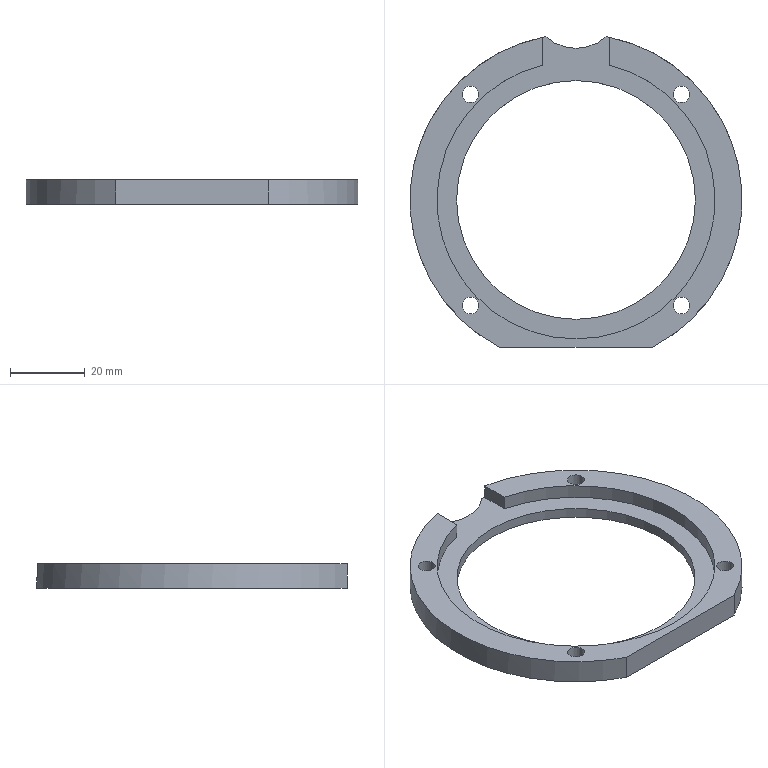Part | NX | features EXTRUDE 3, DATUM_CSYS 1, EXTRACT_DATUM_PLANE 1, SKETCH 1 | 1 solid | 15 faces | box 89 x 83.264 x 6.6 mm | volume 13539 mm3 | cylinder 9 | plane 6 | commonest cylinder face diameters 4.5 x4 89 x2 23.954 x1 64 x1 74.5 x1
STEP:
#1=CARTESIAN_POINT('',(8.062,43.764,2.803));
#2=VERTEX_POINT('',#1);
#3=CARTESIAN_POINT('',(-8.062,43.764,2.803));
#4=VERTEX_POINT('',#3);
#5=CARTESIAN_POINT('',(0.,52.621,2.803));
#6=DIRECTION('',(0.,0.,-1.));
#7=DIRECTION('',(0.6731,-0.7395,0.));
#8=AXIS2_PLACEMENT_3D('',#5,#6,#7);
#9=CIRCLE('',#8,11.977);
#10=EDGE_CURVE('',#2,#4,#9,.T.);
#11=ORIENTED_EDGE('',*,*,#10,.F.);
#12=CARTESIAN_POINT('',(8.062,43.764,0.));
#13=VERTEX_POINT('',#12);
#14=CARTESIAN_POINT('',(8.062,43.764,6.6));
#15=DIRECTION('',(0.,0.,-1.));
#16=VECTOR('',#15,1000.);
#17=LINE('',#14,#16);
#18=EDGE_CURVE('',#2,#13,#17,.T.);
#19=ORIENTED_EDGE('',*,*,#18,.T.);
#20=CARTESIAN_POINT('',(-8.062,43.764,0.));
#21=VERTEX_POINT('',#20);
#22=CARTESIAN_POINT('',(0.,52.621,0.));
#23=DIRECTION('',(0.,0.,-1.));
#24=DIRECTION('',(0.6731,-0.7395,0.));
#25=AXIS2_PLACEMENT_3D('',#22,#23,#24);
#26=CIRCLE('',#25,11.977);
#27=EDGE_CURVE('',#13,#21,#26,.T.);
#28=ORIENTED_EDGE('',*,*,#27,.T.);
#29=CARTESIAN_POINT('',(-8.062,43.764,6.6));
#30=DIRECTION('',(0.,0.,-1.));
#31=VECTOR('',#30,1000.);
#32=LINE('',#29,#31);
#33=EDGE_CURVE('',#4,#21,#32,.T.);
#34=ORIENTED_EDGE('',*,*,#33,.F.);
#35=EDGE_LOOP('',(#11,#19,#28,#34));
#36=FACE_BOUND('',#35,.T.);
#37=CARTESIAN_POINT('',(0.,52.621,6.6));
#38=DIRECTION('',(0.,0.,-1.));
#39=DIRECTION('',(-1.,0.,0.));
#40=AXIS2_PLACEMENT_3D('',#37,#38,#39);
#41=CYLINDRICAL_SURFACE('',#40,11.977);
#42=ADVANCED_FACE('',(#36),#41,.F.);
#43=CARTESIAN_POINT('',(-9.,43.58,2.803));
#44=VERTEX_POINT('',#43);
#45=CARTESIAN_POINT('',(0.,0.,2.803));
#46=DIRECTION('',(0.,0.,1.));
#47=DIRECTION('',(-0.1812,0.9835,0.));
#48=AXIS2_PLACEMENT_3D('',#45,#46,#47);
#49=CIRCLE('',#48,44.5);
#50=EDGE_CURVE('',#4,#44,#49,.T.);
#51=ORIENTED_EDGE('',*,*,#50,.F.);
#52=ORIENTED_EDGE('',*,*,#33,.T.);
#53=CARTESIAN_POINT('',(-20.494,-39.5,0.));
#54=VERTEX_POINT('',#53);
#55=CARTESIAN_POINT('',(0.,0.,0.));
#56=DIRECTION('',(0.,0.,1.));
#57=DIRECTION('',(-0.4605,-0.8876,0.));
#58=AXIS2_PLACEMENT_3D('',#55,#56,#57);
#59=CIRCLE('',#58,44.5);
#60=EDGE_CURVE('',#21,#54,#59,.T.);
#61=ORIENTED_EDGE('',*,*,#60,.T.);
#62=CARTESIAN_POINT('',(-20.494,-39.5,6.6));
#63=VERTEX_POINT('',#62);
#64=CARTESIAN_POINT('',(-20.494,-39.5,6.6));
#65=DIRECTION('',(0.,0.,-1.));
#66=VECTOR('',#65,1000.);
#67=LINE('',#64,#66);
#68=EDGE_CURVE('',#63,#54,#67,.T.);
#69=ORIENTED_EDGE('',*,*,#68,.F.);
#70=CARTESIAN_POINT('',(-9.,43.58,6.6));
#71=VERTEX_POINT('',#70);
#72=CARTESIAN_POINT('',(0.,0.,6.6));
#73=DIRECTION('',(0.,0.,1.));
#74=DIRECTION('',(-1.,0.,0.));
#75=AXIS2_PLACEMENT_3D('',#72,#73,#74);
#76=CIRCLE('',#75,44.5);
#77=EDGE_CURVE('',#71,#63,#76,.T.);
#78=ORIENTED_EDGE('',*,*,#77,.F.);
#79=CARTESIAN_POINT('',(-9.,43.58,27.803));
#80=DIRECTION('',(0.,0.,-1.));
#81=VECTOR('',#80,1000.);
#82=LINE('',#79,#81);
#83=EDGE_CURVE('',#71,#44,#82,.T.);
#84=ORIENTED_EDGE('',*,*,#83,.T.);
#85=EDGE_LOOP('',(#51,#52,#61,#69,#78,#84));
#86=FACE_BOUND('',#85,.T.);
#87=CARTESIAN_POINT('',(0.,0.,6.6));
#88=DIRECTION('',(0.,0.,-1.));
#89=DIRECTION('',(-1.,0.,0.));
#90=AXIS2_PLACEMENT_3D('',#87,#88,#89);
#91=CYLINDRICAL_SURFACE('',#90,44.5);
#92=ADVANCED_FACE('',(#86),#91,.T.);
#93=CARTESIAN_POINT('',(9.,43.58,2.803));
#94=VERTEX_POINT('',#93);
#95=CARTESIAN_POINT('',(0.,0.,2.803));
#96=DIRECTION('',(0.,0.,1.));
#97=DIRECTION('',(0.2022,0.9793,0.));
#98=AXIS2_PLACEMENT_3D('',#95,#96,#97);
#99=CIRCLE('',#98,44.5);
#100=EDGE_CURVE('',#94,#2,#99,.T.);
#101=ORIENTED_EDGE('',*,*,#100,.F.);
#102=CARTESIAN_POINT('',(9.,43.58,6.6));
#103=VERTEX_POINT('',#102);
#104=CARTESIAN_POINT('',(9.,43.58,27.803));
#105=DIRECTION('',(0.,0.,-1.));
#106=VECTOR('',#105,1000.);
#107=LINE('',#104,#106);
#108=EDGE_CURVE('',#103,#94,#107,.T.);
#109=ORIENTED_EDGE('',*,*,#108,.F.);
#110=CARTESIAN_POINT('',(20.494,-39.5,6.6));
#111=VERTEX_POINT('',#110);
#112=CARTESIAN_POINT('',(0.,0.,6.6));
#113=DIRECTION('',(0.,0.,1.));
#114=DIRECTION('',(0.1812,0.9835,0.));
#115=AXIS2_PLACEMENT_3D('',#112,#113,#114);
#116=CIRCLE('',#115,44.5);
#117=EDGE_CURVE('',#111,#103,#116,.T.);
#118=ORIENTED_EDGE('',*,*,#117,.F.);
#119=CARTESIAN_POINT('',(20.494,-39.5,0.));
#120=VERTEX_POINT('',#119);
#121=CARTESIAN_POINT('',(20.494,-39.5,6.6));
#122=DIRECTION('',(0.,0.,-1.));
#123=VECTOR('',#122,1000.);
#124=LINE('',#121,#123);
#125=EDGE_CURVE('',#111,#120,#124,.T.);
#126=ORIENTED_EDGE('',*,*,#125,.T.);
#127=CARTESIAN_POINT('',(0.,0.,0.));
#128=DIRECTION('',(0.,0.,1.));
#129=DIRECTION('',(0.1812,0.9835,0.));
#130=AXIS2_PLACEMENT_3D('',#127,#128,#129);
#131=CIRCLE('',#130,44.5);
#132=EDGE_CURVE('',#120,#13,#131,.T.);
#133=ORIENTED_EDGE('',*,*,#132,.T.);
#134=ORIENTED_EDGE('',*,*,#18,.F.);
#135=EDGE_LOOP('',(#101,#109,#118,#126,#133,#134));
#136=FACE_BOUND('',#135,.T.);
#137=CARTESIAN_POINT('',(0.,0.,6.6));
#138=DIRECTION('',(0.,0.,-1.));
#139=DIRECTION('',(-1.,0.,0.));
#140=AXIS2_PLACEMENT_3D('',#137,#138,#139);
#141=CYLINDRICAL_SURFACE('',#140,44.5);
#142=ADVANCED_FACE('',(#136),#141,.T.);
#143=CARTESIAN_POINT('',(32.,0.,0.));
#144=VERTEX_POINT('',#143);
#145=CARTESIAN_POINT('',(0.,0.,0.));
#146=DIRECTION('',(0.,0.,-1.));
#147=DIRECTION('',(1.,0.,0.));
#148=AXIS2_PLACEMENT_3D('',#145,#146,#147);
#149=CIRCLE('',#148,32.);
#150=EDGE_CURVE('',#144,#144,#149,.T.);
#151=ORIENTED_EDGE('',*,*,#150,.T.);
#152=EDGE_LOOP('',(#151));
#153=FACE_BOUND('',#152,.T.);
#154=CARTESIAN_POINT('',(32.,0.,2.803));
#155=VERTEX_POINT('',#154);
#156=CARTESIAN_POINT('',(0.,0.,2.803));
#157=DIRECTION('',(0.,0.,1.));
#158=DIRECTION('',(1.,0.,0.));
#159=AXIS2_PLACEMENT_3D('',#156,#157,#158);
#160=CIRCLE('',#159,32.);
#161=EDGE_CURVE('',#155,#155,#160,.F.);
#162=ORIENTED_EDGE('',*,*,#161,.F.);
#163=EDGE_LOOP('',(#162));
#164=FACE_BOUND('',#163,.T.);
#165=CARTESIAN_POINT('',(0.,0.,6.6));
#166=DIRECTION('',(0.,0.,-1.));
#167=DIRECTION('',(-1.,0.,0.));
#168=AXIS2_PLACEMENT_3D('',#165,#166,#167);
#169=CYLINDRICAL_SURFACE('',#168,32.);
#170=ADVANCED_FACE('',(#153,#164),#169,.F.);
#171=CARTESIAN_POINT('',(26.034,-28.284,6.6));
#172=VERTEX_POINT('',#171);
#173=CARTESIAN_POINT('',(28.284,-28.284,6.6));
#174=DIRECTION('',(0.,0.,-1.));
#175=DIRECTION('',(-1.,0.,0.));
#176=AXIS2_PLACEMENT_3D('',#173,#174,#175);
#177=CIRCLE('',#176,2.25);
#178=EDGE_CURVE('',#172,#172,#177,.F.);
#179=ORIENTED_EDGE('',*,*,#178,.F.);
#180=EDGE_LOOP('',(#179));
#181=FACE_BOUND('',#180,.T.);
#182=CARTESIAN_POINT('',(-30.534,28.284,6.6));
#183=VERTEX_POINT('',#182);
#184=CARTESIAN_POINT('',(-28.284,28.284,6.6));
#185=DIRECTION('',(0.,0.,-1.));
#186=DIRECTION('',(-1.,0.,0.));
#187=AXIS2_PLACEMENT_3D('',#184,#185,#186);
#188=CIRCLE('',#187,2.25);
#189=EDGE_CURVE('',#183,#183,#188,.F.);
#190=ORIENTED_EDGE('',*,*,#189,.F.);
#191=EDGE_LOOP('',(#190));
#192=FACE_BOUND('',#191,.T.);
#193=CARTESIAN_POINT('',(-30.534,-28.284,6.6));
#194=VERTEX_POINT('',#193);
#195=CARTESIAN_POINT('',(-28.284,-28.284,6.6));
#196=DIRECTION('',(0.,0.,-1.));
#197=DIRECTION('',(-1.,0.,0.));
#198=AXIS2_PLACEMENT_3D('',#195,#196,#197);
#199=CIRCLE('',#198,2.25);
#200=EDGE_CURVE('',#194,#194,#199,.F.);
#201=ORIENTED_EDGE('',*,*,#200,.F.);
#202=EDGE_LOOP('',(#201));
#203=FACE_BOUND('',#202,.T.);
#204=CARTESIAN_POINT('',(26.034,28.284,6.6));
#205=VERTEX_POINT('',#204);
#206=CARTESIAN_POINT('',(28.284,28.284,6.6));
#207=DIRECTION('',(0.,0.,-1.));
#208=DIRECTION('',(-1.,0.,0.));
#209=AXIS2_PLACEMENT_3D('',#206,#207,#208);
#210=CIRCLE('',#209,2.25);
#211=EDGE_CURVE('',#205,#205,#210,.F.);
#212=ORIENTED_EDGE('',*,*,#211,.F.);
#213=EDGE_LOOP('',(#212));
#214=FACE_BOUND('',#213,.T.);
#215=CARTESIAN_POINT('',(-9.,36.146,6.6));
#216=VERTEX_POINT('',#215);
#217=CARTESIAN_POINT('',(-9.,52.621,6.6));
#218=DIRECTION('',(0.,-1.,0.));
#219=VECTOR('',#218,1000.);
#220=LINE('',#217,#219);
#221=EDGE_CURVE('',#71,#216,#220,.T.);
#222=ORIENTED_EDGE('',*,*,#221,.F.);
#223=ORIENTED_EDGE('',*,*,#77,.T.);
#224=CARTESIAN_POINT('',(-20.494,-39.5,6.6));
#225=DIRECTION('',(1.,0.,0.));
#226=VECTOR('',#225,1000.);
#227=LINE('',#224,#226);
#228=EDGE_CURVE('',#63,#111,#227,.T.);
#229=ORIENTED_EDGE('',*,*,#228,.T.);
#230=ORIENTED_EDGE('',*,*,#117,.T.);
#231=CARTESIAN_POINT('',(9.,36.146,6.6));
#232=VERTEX_POINT('',#231);
#233=CARTESIAN_POINT('',(9.,52.621,6.6));
#234=DIRECTION('',(0.,1.,0.));
#235=VECTOR('',#234,1000.);
#236=LINE('',#233,#235);
#237=EDGE_CURVE('',#232,#103,#236,.T.);
#238=ORIENTED_EDGE('',*,*,#237,.F.);
#239=CARTESIAN_POINT('',(0.,0.,6.6));
#240=DIRECTION('',(0.,0.,-1.));
#241=DIRECTION('',(-1.,0.,0.));
#242=AXIS2_PLACEMENT_3D('',#239,#240,#241);
#243=CIRCLE('',#242,37.25);
#244=EDGE_CURVE('',#216,#232,#243,.F.);
#245=ORIENTED_EDGE('',*,*,#244,.F.);
#246=EDGE_LOOP('',(#222,#223,#229,#230,#238,#245));
#247=FACE_BOUND('',#246,.T.);
#248=CARTESIAN_POINT('',(0.,52.621,6.6));
#249=DIRECTION('',(0.,0.,-1.));
#250=DIRECTION('',(-1.,0.,0.));
#251=AXIS2_PLACEMENT_3D('',#248,#249,#250);
#252=PLANE('',#251);
#253=ADVANCED_FACE('',(#181,#192,#203,#214,#247),#252,.F.);
#254=CARTESIAN_POINT('',(-20.494,-39.5,0.));
#255=DIRECTION('',(1.,0.,0.));
#256=VECTOR('',#255,1000.);
#257=LINE('',#254,#256);
#258=EDGE_CURVE('',#54,#120,#257,.T.);
#259=ORIENTED_EDGE('',*,*,#258,.T.);
#260=ORIENTED_EDGE('',*,*,#125,.F.);
#261=ORIENTED_EDGE('',*,*,#228,.F.);
#262=ORIENTED_EDGE('',*,*,#68,.T.);
#263=EDGE_LOOP('',(#259,#260,#261,#262));
#264=FACE_BOUND('',#263,.T.);
#265=CARTESIAN_POINT('',(-20.494,-39.5,6.6));
#266=DIRECTION('',(0.,1.,0.));
#267=DIRECTION('',(0.,0.,1.));
#268=AXIS2_PLACEMENT_3D('',#265,#266,#267);
#269=PLANE('',#268);
#270=ADVANCED_FACE('',(#264),#269,.F.);
#271=CARTESIAN_POINT('',(26.034,-28.284,0.));
#272=VERTEX_POINT('',#271);
#273=CARTESIAN_POINT('',(28.284,-28.284,0.));
#274=DIRECTION('',(0.,0.,-1.));
#275=DIRECTION('',(-1.,0.,0.));
#276=AXIS2_PLACEMENT_3D('',#273,#274,#275);
#277=CIRCLE('',#276,2.25);
#278=EDGE_CURVE('',#272,#272,#277,.F.);
#279=ORIENTED_EDGE('',*,*,#278,.T.);
#280=EDGE_LOOP('',(#279));
#281=FACE_BOUND('',#280,.T.);
#282=CARTESIAN_POINT('',(-30.534,28.284,0.));
#283=VERTEX_POINT('',#282);
#284=CARTESIAN_POINT('',(-28.284,28.284,0.));
#285=DIRECTION('',(0.,0.,-1.));
#286=DIRECTION('',(-1.,0.,0.));
#287=AXIS2_PLACEMENT_3D('',#284,#285,#286);
#288=CIRCLE('',#287,2.25);
#289=EDGE_CURVE('',#283,#283,#288,.F.);
#290=ORIENTED_EDGE('',*,*,#289,.T.);
#291=EDGE_LOOP('',(#290));
#292=FACE_BOUND('',#291,.T.);
#293=CARTESIAN_POINT('',(-30.534,-28.284,0.));
#294=VERTEX_POINT('',#293);
#295=CARTESIAN_POINT('',(-28.284,-28.284,0.));
#296=DIRECTION('',(0.,0.,-1.));
#297=DIRECTION('',(-1.,0.,0.));
#298=AXIS2_PLACEMENT_3D('',#295,#296,#297);
#299=CIRCLE('',#298,2.25);
#300=EDGE_CURVE('',#294,#294,#299,.F.);
#301=ORIENTED_EDGE('',*,*,#300,.T.);
#302=EDGE_LOOP('',(#301));
#303=FACE_BOUND('',#302,.T.);
#304=CARTESIAN_POINT('',(26.034,28.284,0.));
#305=VERTEX_POINT('',#304);
#306=CARTESIAN_POINT('',(28.284,28.284,0.));
#307=DIRECTION('',(0.,0.,-1.));
#308=DIRECTION('',(-1.,0.,0.));
#309=AXIS2_PLACEMENT_3D('',#306,#307,#308);
#310=CIRCLE('',#309,2.25);
#311=EDGE_CURVE('',#305,#305,#310,.F.);
#312=ORIENTED_EDGE('',*,*,#311,.T.);
#313=EDGE_LOOP('',(#312));
#314=FACE_BOUND('',#313,.T.);
#315=ORIENTED_EDGE('',*,*,#27,.F.);
#316=ORIENTED_EDGE('',*,*,#132,.F.);
#317=ORIENTED_EDGE('',*,*,#258,.F.);
#318=ORIENTED_EDGE('',*,*,#60,.F.);
#319=EDGE_LOOP('',(#315,#316,#317,#318));
#320=FACE_BOUND('',#319,.T.);
#321=ORIENTED_EDGE('',*,*,#150,.F.);
#322=EDGE_LOOP('',(#321));
#323=FACE_BOUND('',#322,.T.);
#324=CARTESIAN_POINT('',(0.,52.621,0.));
#325=DIRECTION('',(0.,0.,-1.));
#326=DIRECTION('',(-1.,0.,0.));
#327=AXIS2_PLACEMENT_3D('',#324,#325,#326);
#328=PLANE('',#327);
#329=ADVANCED_FACE('',(#281,#292,#303,#314,#320,#323),#328,.T.);
#330=ORIENTED_EDGE('',*,*,#50,.T.);
#331=CARTESIAN_POINT('',(-9.,36.146,2.803));
#332=VERTEX_POINT('',#331);
#333=CARTESIAN_POINT('',(-9.,43.58,2.803));
#334=DIRECTION('',(0.,-1.,0.));
#335=VECTOR('',#334,1000.);
#336=LINE('',#333,#335);
#337=EDGE_CURVE('',#332,#44,#336,.F.);
#338=ORIENTED_EDGE('',*,*,#337,.F.);
#339=CARTESIAN_POINT('',(9.,36.146,2.803));
#340=VERTEX_POINT('',#339);
#341=CARTESIAN_POINT('',(0.,0.,2.803));
#342=DIRECTION('',(0.,0.,1.));
#343=DIRECTION('',(1.,0.,0.));
#344=AXIS2_PLACEMENT_3D('',#341,#342,#343);
#345=CIRCLE('',#344,37.25);
#346=EDGE_CURVE('',#340,#332,#345,.F.);
#347=ORIENTED_EDGE('',*,*,#346,.F.);
#348=CARTESIAN_POINT('',(9.,36.146,2.803));
#349=DIRECTION('',(0.,1.,0.));
#350=VECTOR('',#349,1000.);
#351=LINE('',#348,#350);
#352=EDGE_CURVE('',#94,#340,#351,.F.);
#353=ORIENTED_EDGE('',*,*,#352,.F.);
#354=ORIENTED_EDGE('',*,*,#100,.T.);
#355=ORIENTED_EDGE('',*,*,#10,.T.);
#356=EDGE_LOOP('',(#330,#338,#347,#353,#354,#355));
#357=FACE_BOUND('',#356,.T.);
#358=ORIENTED_EDGE('',*,*,#161,.T.);
#359=EDGE_LOOP('',(#358));
#360=FACE_BOUND('',#359,.T.);
#361=CARTESIAN_POINT('',(0.,0.,2.803));
#362=DIRECTION('',(0.,0.,1.));
#363=DIRECTION('',(1.,0.,0.));
#364=AXIS2_PLACEMENT_3D('',#361,#362,#363);
#365=PLANE('',#364);
#366=ADVANCED_FACE('',(#357,#360),#365,.T.);
#367=ORIENTED_EDGE('',*,*,#221,.T.);
#368=CARTESIAN_POINT('',(-9.,36.146,27.803));
#369=DIRECTION('',(0.,0.,-1.));
#370=VECTOR('',#369,1000.);
#371=LINE('',#368,#370);
#372=EDGE_CURVE('',#332,#216,#371,.F.);
#373=ORIENTED_EDGE('',*,*,#372,.F.);
#374=ORIENTED_EDGE('',*,*,#337,.T.);
#375=ORIENTED_EDGE('',*,*,#83,.F.);
#376=EDGE_LOOP('',(#367,#373,#374,#375));
#377=FACE_BOUND('',#376,.T.);
#378=CARTESIAN_POINT('',(-9.,43.58,27.803));
#379=DIRECTION('',(1.,0.,0.));
#380=DIRECTION('',(0.,0.,-1.));
#381=AXIS2_PLACEMENT_3D('',#378,#379,#380);
#382=PLANE('',#381);
#383=ADVANCED_FACE('',(#377),#382,.T.);
#384=ORIENTED_EDGE('',*,*,#244,.T.);
#385=CARTESIAN_POINT('',(9.,36.146,27.803));
#386=DIRECTION('',(0.,0.,-1.));
#387=VECTOR('',#386,1000.);
#388=LINE('',#385,#387);
#389=EDGE_CURVE('',#340,#232,#388,.F.);
#390=ORIENTED_EDGE('',*,*,#389,.F.);
#391=ORIENTED_EDGE('',*,*,#346,.T.);
#392=ORIENTED_EDGE('',*,*,#372,.T.);
#393=EDGE_LOOP('',(#384,#390,#391,#392));
#394=FACE_BOUND('',#393,.T.);
#395=CARTESIAN_POINT('',(0.,0.,27.803));
#396=DIRECTION('',(0.,0.,-1.));
#397=DIRECTION('',(-1.,0.,0.));
#398=AXIS2_PLACEMENT_3D('',#395,#396,#397);
#399=CYLINDRICAL_SURFACE('',#398,37.25);
#400=ADVANCED_FACE('',(#394),#399,.F.);
#401=ORIENTED_EDGE('',*,*,#237,.T.);
#402=ORIENTED_EDGE('',*,*,#108,.T.);
#403=ORIENTED_EDGE('',*,*,#352,.T.);
#404=ORIENTED_EDGE('',*,*,#389,.T.);
#405=EDGE_LOOP('',(#401,#402,#403,#404));
#406=FACE_BOUND('',#405,.T.);
#407=CARTESIAN_POINT('',(9.,36.146,27.803));
#408=DIRECTION('',(-1.,0.,0.));
#409=DIRECTION('',(0.,0.,1.));
#410=AXIS2_PLACEMENT_3D('',#407,#408,#409);
#411=PLANE('',#410);
#412=ADVANCED_FACE('',(#406),#411,.T.);
#413=ORIENTED_EDGE('',*,*,#311,.F.);
#414=EDGE_LOOP('',(#413));
#415=FACE_BOUND('',#414,.T.);
#416=ORIENTED_EDGE('',*,*,#211,.T.);
#417=EDGE_LOOP('',(#416));
#418=FACE_BOUND('',#417,.T.);
#419=CARTESIAN_POINT('',(28.284,28.284,27.803));
#420=DIRECTION('',(0.,0.,-1.));
#421=DIRECTION('',(-1.,0.,0.));
#422=AXIS2_PLACEMENT_3D('',#419,#420,#421);
#423=CYLINDRICAL_SURFACE('',#422,2.25);
#424=ADVANCED_FACE('',(#415,#418),#423,.F.);
#425=ORIENTED_EDGE('',*,*,#300,.F.);
#426=EDGE_LOOP('',(#425));
#427=FACE_BOUND('',#426,.T.);
#428=ORIENTED_EDGE('',*,*,#200,.T.);
#429=EDGE_LOOP('',(#428));
#430=FACE_BOUND('',#429,.T.);
#431=CARTESIAN_POINT('',(-28.284,-28.284,27.803));
#432=DIRECTION('',(0.,0.,-1.));
#433=DIRECTION('',(-1.,0.,0.));
#434=AXIS2_PLACEMENT_3D('',#431,#432,#433);
#435=CYLINDRICAL_SURFACE('',#434,2.25);
#436=ADVANCED_FACE('',(#427,#430),#435,.F.);
#437=ORIENTED_EDGE('',*,*,#289,.F.);
#438=EDGE_LOOP('',(#437));
#439=FACE_BOUND('',#438,.T.);
#440=ORIENTED_EDGE('',*,*,#189,.T.);
#441=EDGE_LOOP('',(#440));
#442=FACE_BOUND('',#441,.T.);
#443=CARTESIAN_POINT('',(-28.284,28.284,27.803));
#444=DIRECTION('',(0.,0.,-1.));
#445=DIRECTION('',(-1.,0.,0.));
#446=AXIS2_PLACEMENT_3D('',#443,#444,#445);
#447=CYLINDRICAL_SURFACE('',#446,2.25);
#448=ADVANCED_FACE('',(#439,#442),#447,.F.);
#449=ORIENTED_EDGE('',*,*,#278,.F.);
#450=EDGE_LOOP('',(#449));
#451=FACE_BOUND('',#450,.T.);
#452=ORIENTED_EDGE('',*,*,#178,.T.);
#453=EDGE_LOOP('',(#452));
#454=FACE_BOUND('',#453,.T.);
#455=CARTESIAN_POINT('',(28.284,-28.284,27.803));
#456=DIRECTION('',(0.,0.,-1.));
#457=DIRECTION('',(-1.,0.,0.));
#458=AXIS2_PLACEMENT_3D('',#455,#456,#457);
#459=CYLINDRICAL_SURFACE('',#458,2.25);
#460=ADVANCED_FACE('',(#451,#454),#459,.F.);
#461=CLOSED_SHELL('',(#42,#92,#142,#170,#253,#270,#329,#366,#383,#400,#412,#424,#436,#448,#460));
#462=MANIFOLD_SOLID_BREP('',#461);
#463=(LENGTH_UNIT()NAMED_UNIT(*)SI_UNIT(.MILLI.,.METRE.));
#464=UNCERTAINTY_MEASURE_WITH_UNIT(LENGTH_MEASURE(0.00001),#463,'','');
#465=(NAMED_UNIT(*)PLANE_ANGLE_UNIT()SI_UNIT($,.RADIAN.));
#466=(NAMED_UNIT(*)SI_UNIT($,.STERADIAN.)SOLID_ANGLE_UNIT());
#467=(GEOMETRIC_REPRESENTATION_CONTEXT(3)GLOBAL_UNCERTAINTY_ASSIGNED_CONTEXT((#464))GLOBAL_UNIT_ASSIGNED_CONTEXT((#463,#465,#466))REPRESENTATION_CONTEXT('',''));
#468=ADVANCED_BREP_SHAPE_REPRESENTATION('',(#462),#467);